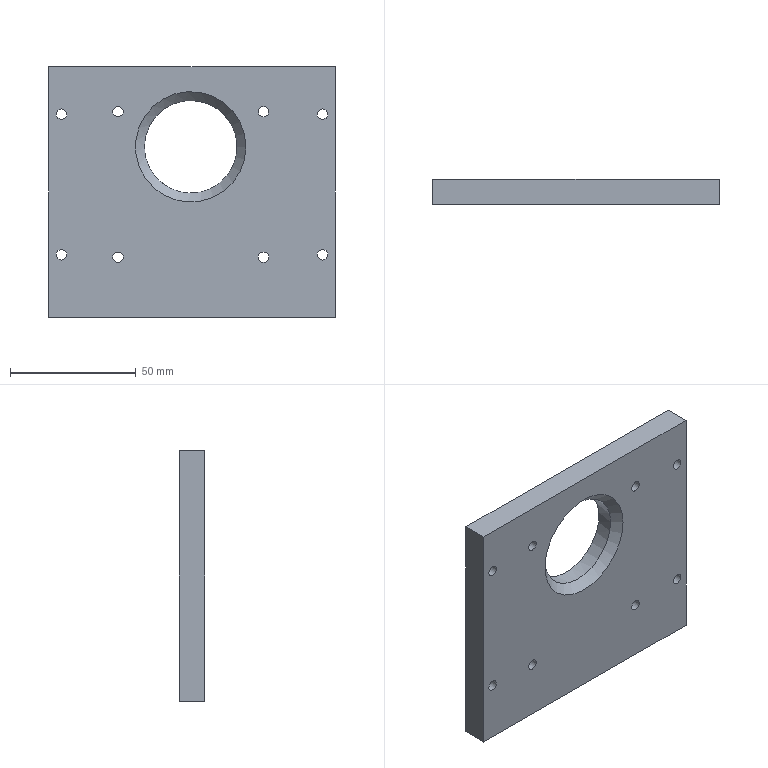Part | STEP file | ROTATION MC_NEW VER-0610_980 | 1 solid | 18 faces | box 114 x 10 x 100 mm | volume 101269 mm3 | cylinder 10 | plane 6 | cone 2 | commonest cylinder face diameters 4.134 x4 4.2 x4 3.3 x1 37 x1
STEP:
#1=CARTESIAN_POINT('',(-288.528,683.508,-245.083));
#2=VERTEX_POINT('',#1);
#3=CARTESIAN_POINT('',(-286.461,683.508,-245.083));
#4=DIRECTION('',(0.,-1.,0.));
#5=DIRECTION('',(1.,0.,0.));
#6=AXIS2_PLACEMENT_3D('',#3,#4,#5);
#7=CIRCLE('',#6,2.067);
#8=EDGE_CURVE('',#2,#2,#7,.T.);
#9=ORIENTED_EDGE('',*,*,#8,.F.);
#10=CARTESIAN_POINT('',(-288.528,673.508,-245.083));
#11=VERTEX_POINT('',#10);
#12=CARTESIAN_POINT('',(-288.528,825.482,-245.083));
#13=DIRECTION('',(0.,-1.,0.));
#14=VECTOR('',#13,2.067);
#15=LINE('',#12,#14);
#16=EDGE_CURVE('',#2,#11,#15,.T.);
#17=ORIENTED_EDGE('',*,*,#16,.T.);
#18=CARTESIAN_POINT('',(-284.394,673.508,-245.083));
#19=VERTEX_POINT('',#18);
#20=CARTESIAN_POINT('',(-286.461,673.508,-245.083));
#21=DIRECTION('',(0.,1.,0.));
#22=DIRECTION('',(1.,0.,0.));
#23=AXIS2_PLACEMENT_3D('',#20,#21,#22);
#24=CIRCLE('',#23,2.067);
#25=EDGE_CURVE('',#19,#11,#24,.T.);
#26=ORIENTED_EDGE('',*,*,#25,.F.);
#27=CARTESIAN_POINT('',(-286.461,673.508,-245.083));
#28=DIRECTION('',(0.,1.,0.));
#29=DIRECTION('',(1.,0.,0.));
#30=AXIS2_PLACEMENT_3D('',#27,#28,#29);
#31=CIRCLE('',#30,2.067);
#32=EDGE_CURVE('',#11,#19,#31,.T.);
#33=ORIENTED_EDGE('',*,*,#32,.F.);
#34=ORIENTED_EDGE('',*,*,#16,.F.);
#35=EDGE_LOOP('',(#9,#17,#26,#33,#34));
#36=FACE_OUTER_BOUND('',#35,.T.);
#37=CARTESIAN_POINT('',(-286.461,825.482,-245.083));
#38=DIRECTION('',(0.,-1.,0.));
#39=DIRECTION('',(1.,0.,0.));
#40=AXIS2_PLACEMENT_3D('',#37,#38,#39);
#41=CYLINDRICAL_SURFACE('',#40,2.067);
#42=ADVANCED_FACE('',(#36),#41,.F.);
#43=CARTESIAN_POINT('',(-288.528,683.508,-187.1));
#44=VERTEX_POINT('',#43);
#45=CARTESIAN_POINT('',(-286.461,683.508,-187.1));
#46=DIRECTION('',(0.,-1.,0.));
#47=DIRECTION('',(1.,0.,0.));
#48=AXIS2_PLACEMENT_3D('',#45,#46,#47);
#49=CIRCLE('',#48,2.067);
#50=EDGE_CURVE('',#44,#44,#49,.T.);
#51=ORIENTED_EDGE('',*,*,#50,.F.);
#52=CARTESIAN_POINT('',(-288.528,673.508,-187.1));
#53=VERTEX_POINT('',#52);
#54=CARTESIAN_POINT('',(-288.528,825.482,-187.1));
#55=DIRECTION('',(0.,-1.,0.));
#56=VECTOR('',#55,2.067);
#57=LINE('',#54,#56);
#58=EDGE_CURVE('',#44,#53,#57,.T.);
#59=ORIENTED_EDGE('',*,*,#58,.T.);
#60=CARTESIAN_POINT('',(-284.394,673.508,-187.1));
#61=VERTEX_POINT('',#60);
#62=CARTESIAN_POINT('',(-286.461,673.508,-187.1));
#63=DIRECTION('',(0.,1.,0.));
#64=DIRECTION('',(1.,0.,0.));
#65=AXIS2_PLACEMENT_3D('',#62,#63,#64);
#66=CIRCLE('',#65,2.067);
#67=EDGE_CURVE('',#61,#53,#66,.T.);
#68=ORIENTED_EDGE('',*,*,#67,.F.);
#69=CARTESIAN_POINT('',(-286.461,673.508,-187.1));
#70=DIRECTION('',(0.,1.,0.));
#71=DIRECTION('',(1.,0.,0.));
#72=AXIS2_PLACEMENT_3D('',#69,#70,#71);
#73=CIRCLE('',#72,2.067);
#74=EDGE_CURVE('',#53,#61,#73,.T.);
#75=ORIENTED_EDGE('',*,*,#74,.F.);
#76=ORIENTED_EDGE('',*,*,#58,.F.);
#77=EDGE_LOOP('',(#51,#59,#68,#75,#76));
#78=FACE_OUTER_BOUND('',#77,.T.);
#79=CARTESIAN_POINT('',(-286.461,825.482,-187.1));
#80=DIRECTION('',(0.,-1.,0.));
#81=DIRECTION('',(1.,0.,0.));
#82=AXIS2_PLACEMENT_3D('',#79,#80,#81);
#83=CYLINDRICAL_SURFACE('',#82,2.067);
#84=ADVANCED_FACE('',(#78),#83,.F.);
#85=CARTESIAN_POINT('',(-230.545,683.508,-187.1));
#86=VERTEX_POINT('',#85);
#87=CARTESIAN_POINT('',(-228.478,683.508,-187.1));
#88=DIRECTION('',(0.,-1.,0.));
#89=DIRECTION('',(1.,0.,0.));
#90=AXIS2_PLACEMENT_3D('',#87,#88,#89);
#91=CIRCLE('',#90,2.067);
#92=EDGE_CURVE('',#86,#86,#91,.T.);
#93=ORIENTED_EDGE('',*,*,#92,.F.);
#94=CARTESIAN_POINT('',(-230.545,673.508,-187.1));
#95=VERTEX_POINT('',#94);
#96=CARTESIAN_POINT('',(-230.545,825.482,-187.1));
#97=DIRECTION('',(0.,-1.,0.));
#98=VECTOR('',#97,2.067);
#99=LINE('',#96,#98);
#100=EDGE_CURVE('',#86,#95,#99,.T.);
#101=ORIENTED_EDGE('',*,*,#100,.T.);
#102=CARTESIAN_POINT('',(-226.411,673.508,-187.1));
#103=VERTEX_POINT('',#102);
#104=CARTESIAN_POINT('',(-228.478,673.508,-187.1));
#105=DIRECTION('',(0.,1.,0.));
#106=DIRECTION('',(1.,0.,0.));
#107=AXIS2_PLACEMENT_3D('',#104,#105,#106);
#108=CIRCLE('',#107,2.067);
#109=EDGE_CURVE('',#103,#95,#108,.T.);
#110=ORIENTED_EDGE('',*,*,#109,.F.);
#111=CARTESIAN_POINT('',(-228.478,673.508,-187.1));
#112=DIRECTION('',(0.,1.,0.));
#113=DIRECTION('',(1.,0.,0.));
#114=AXIS2_PLACEMENT_3D('',#111,#112,#113);
#115=CIRCLE('',#114,2.067);
#116=EDGE_CURVE('',#95,#103,#115,.T.);
#117=ORIENTED_EDGE('',*,*,#116,.F.);
#118=ORIENTED_EDGE('',*,*,#100,.F.);
#119=EDGE_LOOP('',(#93,#101,#110,#117,#118));
#120=FACE_OUTER_BOUND('',#119,.T.);
#121=CARTESIAN_POINT('',(-228.478,825.482,-187.1));
#122=DIRECTION('',(0.,-1.,0.));
#123=DIRECTION('',(1.,0.,0.));
#124=AXIS2_PLACEMENT_3D('',#121,#122,#123);
#125=CYLINDRICAL_SURFACE('',#124,2.067);
#126=ADVANCED_FACE('',(#120),#125,.F.);
#127=CARTESIAN_POINT('',(-230.545,683.508,-245.083));
#128=VERTEX_POINT('',#127);
#129=CARTESIAN_POINT('',(-228.478,683.508,-245.083));
#130=DIRECTION('',(0.,-1.,0.));
#131=DIRECTION('',(1.,0.,0.));
#132=AXIS2_PLACEMENT_3D('',#129,#130,#131);
#133=CIRCLE('',#132,2.067);
#134=EDGE_CURVE('',#128,#128,#133,.T.);
#135=ORIENTED_EDGE('',*,*,#134,.F.);
#136=CARTESIAN_POINT('',(-230.545,673.508,-245.083));
#137=VERTEX_POINT('',#136);
#138=CARTESIAN_POINT('',(-230.545,825.482,-245.083));
#139=DIRECTION('',(0.,-1.,0.));
#140=VECTOR('',#139,2.067);
#141=LINE('',#138,#140);
#142=EDGE_CURVE('',#128,#137,#141,.T.);
#143=ORIENTED_EDGE('',*,*,#142,.T.);
#144=CARTESIAN_POINT('',(-226.411,673.508,-245.083));
#145=VERTEX_POINT('',#144);
#146=CARTESIAN_POINT('',(-228.478,673.508,-245.083));
#147=DIRECTION('',(0.,1.,0.));
#148=DIRECTION('',(1.,0.,0.));
#149=AXIS2_PLACEMENT_3D('',#146,#147,#148);
#150=CIRCLE('',#149,2.067);
#151=EDGE_CURVE('',#145,#137,#150,.T.);
#152=ORIENTED_EDGE('',*,*,#151,.F.);
#153=CARTESIAN_POINT('',(-228.478,673.508,-245.083));
#154=DIRECTION('',(0.,1.,0.));
#155=DIRECTION('',(1.,0.,0.));
#156=AXIS2_PLACEMENT_3D('',#153,#154,#155);
#157=CIRCLE('',#156,2.067);
#158=EDGE_CURVE('',#137,#145,#157,.T.);
#159=ORIENTED_EDGE('',*,*,#158,.F.);
#160=ORIENTED_EDGE('',*,*,#142,.F.);
#161=EDGE_LOOP('',(#135,#143,#152,#159,#160));
#162=FACE_OUTER_BOUND('',#161,.T.);
#163=CARTESIAN_POINT('',(-228.478,825.482,-245.083));
#164=DIRECTION('',(0.,-1.,0.));
#165=DIRECTION('',(1.,0.,0.));
#166=AXIS2_PLACEMENT_3D('',#163,#164,#165);
#167=CYLINDRICAL_SURFACE('',#166,2.067);
#168=ADVANCED_FACE('',(#162),#167,.F.);
#169=CARTESIAN_POINT('',(-308.969,683.508,-185.991));
#170=VERTEX_POINT('',#169);
#171=CARTESIAN_POINT('',(-308.969,683.508,-188.091));
#172=DIRECTION('',(0.,1.,0.));
#173=DIRECTION('',(0.,0.,1.));
#174=AXIS2_PLACEMENT_3D('',#171,#172,#173);
#175=CIRCLE('',#174,2.1);
#176=EDGE_CURVE('',#170,#170,#175,.F.);
#177=ORIENTED_EDGE('',*,*,#176,.F.);
#178=CARTESIAN_POINT('',(-308.969,673.508,-185.991));
#179=VERTEX_POINT('',#178);
#180=CARTESIAN_POINT('',(-308.969,683.508,-185.991));
#181=DIRECTION('',(0.,-1.,0.));
#182=VECTOR('',#181,2.1);
#183=LINE('',#180,#182);
#184=EDGE_CURVE('',#170,#179,#183,.T.);
#185=ORIENTED_EDGE('',*,*,#184,.T.);
#186=CARTESIAN_POINT('',(-308.969,673.508,-188.091));
#187=DIRECTION('',(0.,1.,0.));
#188=DIRECTION('',(0.,0.,1.));
#189=AXIS2_PLACEMENT_3D('',#186,#187,#188);
#190=CIRCLE('',#189,2.1);
#191=EDGE_CURVE('',#179,#179,#190,.T.);
#192=ORIENTED_EDGE('',*,*,#191,.F.);
#193=ORIENTED_EDGE('',*,*,#184,.F.);
#194=EDGE_LOOP('',(#177,#185,#192,#193));
#195=FACE_OUTER_BOUND('',#194,.T.);
#196=CARTESIAN_POINT('',(-308.969,683.508,-188.091));
#197=DIRECTION('',(0.,-1.,0.));
#198=DIRECTION('',(0.,0.,-1.));
#199=AXIS2_PLACEMENT_3D('',#196,#197,#198);
#200=CYLINDRICAL_SURFACE('',#199,2.1);
#201=ADVANCED_FACE('',(#195),#200,.F.);
#202=CARTESIAN_POINT('',(-308.969,683.508,-241.991));
#203=VERTEX_POINT('',#202);
#204=CARTESIAN_POINT('',(-308.969,683.508,-244.091));
#205=DIRECTION('',(0.,1.,0.));
#206=DIRECTION('',(0.,0.,1.));
#207=AXIS2_PLACEMENT_3D('',#204,#205,#206);
#208=CIRCLE('',#207,2.1);
#209=EDGE_CURVE('',#203,#203,#208,.F.);
#210=ORIENTED_EDGE('',*,*,#209,.F.);
#211=CARTESIAN_POINT('',(-308.969,673.508,-241.991));
#212=VERTEX_POINT('',#211);
#213=CARTESIAN_POINT('',(-308.969,683.508,-241.991));
#214=DIRECTION('',(0.,-1.,0.));
#215=VECTOR('',#214,2.1);
#216=LINE('',#213,#215);
#217=EDGE_CURVE('',#203,#212,#216,.T.);
#218=ORIENTED_EDGE('',*,*,#217,.T.);
#219=CARTESIAN_POINT('',(-308.969,673.508,-244.091));
#220=DIRECTION('',(0.,1.,0.));
#221=DIRECTION('',(0.,0.,1.));
#222=AXIS2_PLACEMENT_3D('',#219,#220,#221);
#223=CIRCLE('',#222,2.1);
#224=EDGE_CURVE('',#212,#212,#223,.T.);
#225=ORIENTED_EDGE('',*,*,#224,.F.);
#226=ORIENTED_EDGE('',*,*,#217,.F.);
#227=EDGE_LOOP('',(#210,#218,#225,#226));
#228=FACE_OUTER_BOUND('',#227,.T.);
#229=CARTESIAN_POINT('',(-308.969,683.508,-244.091));
#230=DIRECTION('',(0.,-1.,0.));
#231=DIRECTION('',(0.,0.,-1.));
#232=AXIS2_PLACEMENT_3D('',#229,#230,#231);
#233=CYLINDRICAL_SURFACE('',#232,2.1);
#234=ADVANCED_FACE('',(#228),#233,.F.);
#235=CARTESIAN_POINT('',(-204.969,683.508,-241.991));
#236=VERTEX_POINT('',#235);
#237=CARTESIAN_POINT('',(-204.969,683.508,-244.091));
#238=DIRECTION('',(0.,1.,0.));
#239=DIRECTION('',(0.,0.,1.));
#240=AXIS2_PLACEMENT_3D('',#237,#238,#239);
#241=CIRCLE('',#240,2.1);
#242=EDGE_CURVE('',#236,#236,#241,.F.);
#243=ORIENTED_EDGE('',*,*,#242,.F.);
#244=CARTESIAN_POINT('',(-204.969,673.508,-241.991));
#245=VERTEX_POINT('',#244);
#246=CARTESIAN_POINT('',(-204.969,683.508,-241.991));
#247=DIRECTION('',(0.,-1.,0.));
#248=VECTOR('',#247,2.1);
#249=LINE('',#246,#248);
#250=EDGE_CURVE('',#236,#245,#249,.T.);
#251=ORIENTED_EDGE('',*,*,#250,.T.);
#252=CARTESIAN_POINT('',(-204.969,673.508,-244.091));
#253=DIRECTION('',(0.,1.,0.));
#254=DIRECTION('',(0.,0.,1.));
#255=AXIS2_PLACEMENT_3D('',#252,#253,#254);
#256=CIRCLE('',#255,2.1);
#257=EDGE_CURVE('',#245,#245,#256,.T.);
#258=ORIENTED_EDGE('',*,*,#257,.F.);
#259=ORIENTED_EDGE('',*,*,#250,.F.);
#260=EDGE_LOOP('',(#243,#251,#258,#259));
#261=FACE_OUTER_BOUND('',#260,.T.);
#262=CARTESIAN_POINT('',(-204.969,683.508,-244.091));
#263=DIRECTION('',(0.,-1.,0.));
#264=DIRECTION('',(0.,0.,-1.));
#265=AXIS2_PLACEMENT_3D('',#262,#263,#264);
#266=CYLINDRICAL_SURFACE('',#265,2.1);
#267=ADVANCED_FACE('',(#261),#266,.F.);
#268=CARTESIAN_POINT('',(-204.969,683.508,-185.991));
#269=VERTEX_POINT('',#268);
#270=CARTESIAN_POINT('',(-204.969,683.508,-188.091));
#271=DIRECTION('',(0.,1.,0.));
#272=DIRECTION('',(0.,0.,1.));
#273=AXIS2_PLACEMENT_3D('',#270,#271,#272);
#274=CIRCLE('',#273,2.1);
#275=EDGE_CURVE('',#269,#269,#274,.F.);
#276=ORIENTED_EDGE('',*,*,#275,.F.);
#277=CARTESIAN_POINT('',(-204.969,673.508,-185.991));
#278=VERTEX_POINT('',#277);
#279=CARTESIAN_POINT('',(-204.969,683.508,-185.991));
#280=DIRECTION('',(0.,-1.,0.));
#281=VECTOR('',#280,2.1);
#282=LINE('',#279,#281);
#283=EDGE_CURVE('',#269,#278,#282,.T.);
#284=ORIENTED_EDGE('',*,*,#283,.T.);
#285=CARTESIAN_POINT('',(-204.969,673.508,-188.091));
#286=DIRECTION('',(0.,1.,0.));
#287=DIRECTION('',(0.,0.,1.));
#288=AXIS2_PLACEMENT_3D('',#285,#286,#287);
#289=CIRCLE('',#288,2.1);
#290=EDGE_CURVE('',#278,#278,#289,.T.);
#291=ORIENTED_EDGE('',*,*,#290,.F.);
#292=ORIENTED_EDGE('',*,*,#283,.F.);
#293=EDGE_LOOP('',(#276,#284,#291,#292));
#294=FACE_OUTER_BOUND('',#293,.T.);
#295=CARTESIAN_POINT('',(-204.969,683.508,-188.091));
#296=DIRECTION('',(0.,-1.,0.));
#297=DIRECTION('',(0.,0.,-1.));
#298=AXIS2_PLACEMENT_3D('',#295,#296,#297);
#299=CYLINDRICAL_SURFACE('',#298,2.1);
#300=ADVANCED_FACE('',(#294),#299,.F.);
#301=CARTESIAN_POINT('',(-256.969,678.358,-269.091));
#302=VERTEX_POINT('',#301);
#303=CARTESIAN_POINT('',(-256.969,681.658,-269.091));
#304=VERTEX_POINT('',#303);
#305=CARTESIAN_POINT('',(-256.969,680.008,-269.091));
#306=DIRECTION('',(0.,0.,1.));
#307=DIRECTION('',(0.,-1.,0.));
#308=AXIS2_PLACEMENT_3D('',#305,#306,#307);
#309=CIRCLE('',#308,1.65);
#310=EDGE_CURVE('',#302,#304,#309,.T.);
#311=ORIENTED_EDGE('',*,*,#310,.F.);
#312=CARTESIAN_POINT('',(-256.969,680.008,-269.091));
#313=DIRECTION('',(0.,0.,1.));
#314=DIRECTION('',(0.,-1.,0.));
#315=AXIS2_PLACEMENT_3D('',#312,#313,#314);
#316=CIRCLE('',#315,1.65);
#317=EDGE_CURVE('',#304,#302,#316,.T.);
#318=ORIENTED_EDGE('',*,*,#317,.F.);
#319=CARTESIAN_POINT('',(-256.969,681.658,-254.091));
#320=VERTEX_POINT('',#319);
#321=CARTESIAN_POINT('',(-256.969,681.658,-269.091));
#322=DIRECTION('',(0.,0.,1.));
#323=VECTOR('',#322,1.65);
#324=LINE('',#321,#323);
#325=EDGE_CURVE('',#304,#320,#324,.T.);
#326=ORIENTED_EDGE('',*,*,#325,.T.);
#327=CARTESIAN_POINT('',(-256.969,678.358,-254.091));
#328=VERTEX_POINT('',#327);
#329=CARTESIAN_POINT('',(-256.969,680.008,-254.091));
#330=DIRECTION('',(0.,0.,-1.));
#331=DIRECTION('',(0.,-1.,0.));
#332=AXIS2_PLACEMENT_3D('',#329,#330,#331);
#333=CIRCLE('',#332,1.65);
#334=EDGE_CURVE('',#328,#320,#333,.T.);
#335=ORIENTED_EDGE('',*,*,#334,.F.);
#336=CARTESIAN_POINT('',(-256.969,680.008,-254.091));
#337=DIRECTION('',(0.,0.,-1.));
#338=DIRECTION('',(0.,-1.,0.));
#339=AXIS2_PLACEMENT_3D('',#336,#337,#338);
#340=CIRCLE('',#339,1.65);
#341=EDGE_CURVE('',#320,#328,#340,.T.);
#342=ORIENTED_EDGE('',*,*,#341,.F.);
#343=ORIENTED_EDGE('',*,*,#325,.F.);
#344=EDGE_LOOP('',(#311,#318,#326,#335,#342,#343));
#345=FACE_OUTER_BOUND('',#344,.T.);
#346=CARTESIAN_POINT('',(-256.969,680.008,-269.091));
#347=DIRECTION('',(0.,0.,1.));
#348=DIRECTION('',(0.,-1.,0.));
#349=AXIS2_PLACEMENT_3D('',#346,#347,#348);
#350=CYLINDRICAL_SURFACE('',#349,1.65);
#351=ADVANCED_FACE('',(#345),#350,.F.);
#352=CARTESIAN_POINT('',(-256.969,680.008,-253.1));
#353=VERTEX_POINT('',#352);
#354=CARTESIAN_POINT('',(-256.969,678.358,-254.091));
#355=DIRECTION('',(0.,-0.8572,-0.515));
#356=VECTOR('',#355,1.65);
#357=LINE('',#354,#356);
#358=EDGE_CURVE('',#353,#328,#357,.T.);
#359=ORIENTED_EDGE('',*,*,#358,.T.);
#360=ORIENTED_EDGE('',*,*,#334,.T.);
#361=ORIENTED_EDGE('',*,*,#341,.T.);
#362=ORIENTED_EDGE('',*,*,#358,.F.);
#363=EDGE_LOOP('',(#359,#360,#361,#362));
#364=FACE_OUTER_BOUND('',#363,.T.);
#365=CARTESIAN_POINT('',(-256.969,680.008,-254.091));
#366=DIRECTION('',(0.,0.,-1.));
#367=DIRECTION('',(0.,1.,0.));
#368=AXIS2_PLACEMENT_3D('',#365,#366,#367);
#369=CONICAL_SURFACE('',#368,1.65,1.03);
#370=ADVANCED_FACE('',(#364),#369,.F.);
#371=CARTESIAN_POINT('',(-199.969,673.508,-269.091));
#372=VERTEX_POINT('',#371);
#373=CARTESIAN_POINT('',(-313.969,673.508,-269.091));
#374=VERTEX_POINT('',#373);
#375=CARTESIAN_POINT('',(-199.969,673.508,-269.091));
#376=DIRECTION('',(-1.,0.,0.));
#377=VECTOR('',#376,114.);
#378=LINE('',#375,#377);
#379=EDGE_CURVE('',#372,#374,#378,.T.);
#380=ORIENTED_EDGE('',*,*,#379,.T.);
#381=CARTESIAN_POINT('',(-313.969,683.508,-269.091));
#382=VERTEX_POINT('',#381);
#383=CARTESIAN_POINT('',(-313.969,683.508,-269.091));
#384=DIRECTION('',(0.,-1.,0.));
#385=VECTOR('',#384,10.);
#386=LINE('',#383,#385);
#387=EDGE_CURVE('',#382,#374,#386,.T.);
#388=ORIENTED_EDGE('',*,*,#387,.F.);
#389=CARTESIAN_POINT('',(-199.969,683.508,-269.091));
#390=VERTEX_POINT('',#389);
#391=CARTESIAN_POINT('',(-199.969,683.508,-269.091));
#392=DIRECTION('',(-1.,0.,0.));
#393=VECTOR('',#392,114.);
#394=LINE('',#391,#393);
#395=EDGE_CURVE('',#390,#382,#394,.T.);
#396=ORIENTED_EDGE('',*,*,#395,.F.);
#397=CARTESIAN_POINT('',(-199.969,683.508,-269.091));
#398=DIRECTION('',(0.,-1.,0.));
#399=VECTOR('',#398,10.);
#400=LINE('',#397,#399);
#401=EDGE_CURVE('',#390,#372,#400,.T.);
#402=ORIENTED_EDGE('',*,*,#401,.T.);
#403=EDGE_LOOP('',(#380,#388,#396,#402));
#404=FACE_OUTER_BOUND('',#403,.T.);
#405=ORIENTED_EDGE('',*,*,#310,.T.);
#406=ORIENTED_EDGE('',*,*,#317,.T.);
#407=EDGE_LOOP('',(#405,#406));
#408=FACE_BOUND('',#407,.T.);
#409=CARTESIAN_POINT('',(-258.469,676.508,-269.091));
#410=DIRECTION('',(0.,0.,-1.));
#411=DIRECTION('',(-1.,0.,0.));
#412=AXIS2_PLACEMENT_3D('',#409,#410,#411);
#413=PLANE('',#412);
#414=ADVANCED_FACE('',(#404,#408),#413,.T.);
#415=CARTESIAN_POINT('',(-313.969,683.508,-169.091));
#416=VERTEX_POINT('',#415);
#417=CARTESIAN_POINT('',(-313.969,683.508,-269.091));
#418=DIRECTION('',(0.,0.,1.));
#419=VECTOR('',#418,100.);
#420=LINE('',#417,#419);
#421=EDGE_CURVE('',#382,#416,#420,.T.);
#422=ORIENTED_EDGE('',*,*,#421,.T.);
#423=CARTESIAN_POINT('',(-199.969,683.508,-169.091));
#424=VERTEX_POINT('',#423);
#425=CARTESIAN_POINT('',(-199.969,683.508,-169.091));
#426=DIRECTION('',(-1.,0.,0.));
#427=VECTOR('',#426,114.);
#428=LINE('',#425,#427);
#429=EDGE_CURVE('',#424,#416,#428,.T.);
#430=ORIENTED_EDGE('',*,*,#429,.F.);
#431=CARTESIAN_POINT('',(-199.969,683.508,-269.091));
#432=DIRECTION('',(0.,0.,1.));
#433=VECTOR('',#432,100.);
#434=LINE('',#431,#433);
#435=EDGE_CURVE('',#390,#424,#434,.T.);
#436=ORIENTED_EDGE('',*,*,#435,.F.);
#437=ORIENTED_EDGE('',*,*,#395,.T.);
#438=EDGE_LOOP('',(#422,#430,#436,#437));
#439=FACE_OUTER_BOUND('',#438,.T.);
#440=ORIENTED_EDGE('',*,*,#8,.T.);
#441=EDGE_LOOP('',(#440));
#442=FACE_BOUND('',#441,.T.);
#443=ORIENTED_EDGE('',*,*,#50,.T.);
#444=EDGE_LOOP('',(#443));
#445=FACE_BOUND('',#444,.T.);
#446=ORIENTED_EDGE('',*,*,#92,.T.);
#447=EDGE_LOOP('',(#446));
#448=FACE_BOUND('',#447,.T.);
#449=ORIENTED_EDGE('',*,*,#134,.T.);
#450=EDGE_LOOP('',(#449));
#451=FACE_BOUND('',#450,.T.);
#452=ORIENTED_EDGE('',*,*,#275,.T.);
#453=EDGE_LOOP('',(#452));
#454=FACE_BOUND('',#453,.T.);
#455=ORIENTED_EDGE('',*,*,#242,.T.);
#456=EDGE_LOOP('',(#455));
#457=FACE_BOUND('',#456,.T.);
#458=ORIENTED_EDGE('',*,*,#209,.T.);
#459=EDGE_LOOP('',(#458));
#460=FACE_BOUND('',#459,.T.);
#461=ORIENTED_EDGE('',*,*,#176,.T.);
#462=EDGE_LOOP('',(#461));
#463=FACE_BOUND('',#462,.T.);
#464=CARTESIAN_POINT('',(-257.469,683.508,-182.591));
#465=VERTEX_POINT('',#464);
#466=CARTESIAN_POINT('',(-275.969,683.508,-201.091));
#467=VERTEX_POINT('',#466);
#468=CARTESIAN_POINT('',(-257.469,683.508,-201.091));
#469=DIRECTION('',(0.,-1.,0.));
#470=DIRECTION('',(0.,0.,1.));
#471=AXIS2_PLACEMENT_3D('',#468,#469,#470);
#472=CIRCLE('',#471,18.5);
#473=EDGE_CURVE('',#465,#467,#472,.T.);
#474=ORIENTED_EDGE('',*,*,#473,.T.);
#475=CARTESIAN_POINT('',(-257.469,683.508,-201.091));
#476=DIRECTION('',(0.,-1.,0.));
#477=DIRECTION('',(0.,0.,1.));
#478=AXIS2_PLACEMENT_3D('',#475,#476,#477);
#479=CIRCLE('',#478,18.5);
#480=EDGE_CURVE('',#467,#465,#479,.T.);
#481=ORIENTED_EDGE('',*,*,#480,.T.);
#482=EDGE_LOOP('',(#474,#481));
#483=FACE_BOUND('',#482,.T.);
#484=CARTESIAN_POINT('',(-257.469,683.508,-228.812));
#485=DIRECTION('',(0.,1.,0.));
#486=DIRECTION('',(0.,0.,1.));
#487=AXIS2_PLACEMENT_3D('',#484,#485,#486);
#488=PLANE('',#487);
#489=ADVANCED_FACE('',(#439,#442,#445,#448,#451,#454,#457,#460,#463,#483),#488,.T.);
#490=CARTESIAN_POINT('',(-313.969,673.508,-169.091));
#491=VERTEX_POINT('',#490);
#492=CARTESIAN_POINT('',(-199.969,673.508,-169.091));
#493=VERTEX_POINT('',#492);
#494=CARTESIAN_POINT('',(-313.969,673.508,-169.091));
#495=DIRECTION('',(1.,0.,0.));
#496=VECTOR('',#495,114.);
#497=LINE('',#494,#496);
#498=EDGE_CURVE('',#491,#493,#497,.T.);
#499=ORIENTED_EDGE('',*,*,#498,.F.);
#500=CARTESIAN_POINT('',(-313.969,673.508,-269.091));
#501=DIRECTION('',(0.,0.,1.));
#502=VECTOR('',#501,100.);
#503=LINE('',#500,#502);
#504=EDGE_CURVE('',#374,#491,#503,.T.);
#505=ORIENTED_EDGE('',*,*,#504,.F.);
#506=ORIENTED_EDGE('',*,*,#379,.F.);
#507=CARTESIAN_POINT('',(-199.969,673.508,-169.091));
#508=DIRECTION('',(0.,0.,-1.));
#509=VECTOR('',#508,100.);
#510=LINE('',#507,#509);
#511=EDGE_CURVE('',#493,#372,#510,.T.);
#512=ORIENTED_EDGE('',*,*,#511,.F.);
#513=EDGE_LOOP('',(#499,#505,#506,#512));
#514=FACE_OUTER_BOUND('',#513,.T.);
#515=ORIENTED_EDGE('',*,*,#25,.T.);
#516=ORIENTED_EDGE('',*,*,#32,.T.);
#517=EDGE_LOOP('',(#515,#516));
#518=FACE_BOUND('',#517,.T.);
#519=ORIENTED_EDGE('',*,*,#67,.T.);
#520=ORIENTED_EDGE('',*,*,#74,.T.);
#521=EDGE_LOOP('',(#519,#520));
#522=FACE_BOUND('',#521,.T.);
#523=ORIENTED_EDGE('',*,*,#109,.T.);
#524=ORIENTED_EDGE('',*,*,#116,.T.);
#525=EDGE_LOOP('',(#523,#524));
#526=FACE_BOUND('',#525,.T.);
#527=ORIENTED_EDGE('',*,*,#151,.T.);
#528=ORIENTED_EDGE('',*,*,#158,.T.);
#529=EDGE_LOOP('',(#527,#528));
#530=FACE_BOUND('',#529,.T.);
#531=CARTESIAN_POINT('',(-235.469,673.508,-201.091));
#532=VERTEX_POINT('',#531);
#533=CARTESIAN_POINT('',(-257.469,673.508,-201.091));
#534=DIRECTION('',(0.,1.,0.));
#535=DIRECTION('',(-1.,0.,0.));
#536=AXIS2_PLACEMENT_3D('',#533,#534,#535);
#537=CIRCLE('',#536,22.);
#538=EDGE_CURVE('',#532,#532,#537,.T.);
#539=ORIENTED_EDGE('',*,*,#538,.T.);
#540=EDGE_LOOP('',(#539));
#541=FACE_BOUND('',#540,.T.);
#542=ORIENTED_EDGE('',*,*,#290,.T.);
#543=EDGE_LOOP('',(#542));
#544=FACE_BOUND('',#543,.T.);
#545=ORIENTED_EDGE('',*,*,#257,.T.);
#546=EDGE_LOOP('',(#545));
#547=FACE_BOUND('',#546,.T.);
#548=ORIENTED_EDGE('',*,*,#224,.T.);
#549=EDGE_LOOP('',(#548));
#550=FACE_BOUND('',#549,.T.);
#551=ORIENTED_EDGE('',*,*,#191,.T.);
#552=EDGE_LOOP('',(#551));
#553=FACE_BOUND('',#552,.T.);
#554=CARTESIAN_POINT('',(-257.469,673.508,-216.091));
#555=DIRECTION('',(0.,1.,0.));
#556=DIRECTION('',(0.,0.,1.));
#557=AXIS2_PLACEMENT_3D('',#554,#555,#556);
#558=PLANE('',#557);
#559=ADVANCED_FACE('',(#514,#518,#522,#526,#530,#541,#544,#547,#550,#553),#558,.F.);
#560=ORIENTED_EDGE('',*,*,#421,.F.);
#561=ORIENTED_EDGE('',*,*,#387,.T.);
#562=ORIENTED_EDGE('',*,*,#504,.T.);
#563=CARTESIAN_POINT('',(-313.969,673.508,-169.091));
#564=DIRECTION('',(0.,1.,0.));
#565=VECTOR('',#564,10.);
#566=LINE('',#563,#565);
#567=EDGE_CURVE('',#491,#416,#566,.T.);
#568=ORIENTED_EDGE('',*,*,#567,.T.);
#569=EDGE_LOOP('',(#560,#561,#562,#568));
#570=FACE_OUTER_BOUND('',#569,.T.);
#571=CARTESIAN_POINT('',(-313.969,676.508,-228.812));
#572=DIRECTION('',(-1.,0.,0.));
#573=DIRECTION('',(0.,0.,1.));
#574=AXIS2_PLACEMENT_3D('',#571,#572,#573);
#575=PLANE('',#574);
#576=ADVANCED_FACE('',(#570),#575,.T.);
#577=ORIENTED_EDGE('',*,*,#498,.T.);
#578=CARTESIAN_POINT('',(-199.969,673.508,-169.091));
#579=DIRECTION('',(0.,1.,0.));
#580=VECTOR('',#579,10.);
#581=LINE('',#578,#580);
#582=EDGE_CURVE('',#493,#424,#581,.T.);
#583=ORIENTED_EDGE('',*,*,#582,.T.);
#584=ORIENTED_EDGE('',*,*,#429,.T.);
#585=ORIENTED_EDGE('',*,*,#567,.F.);
#586=EDGE_LOOP('',(#577,#583,#584,#585));
#587=FACE_OUTER_BOUND('',#586,.T.);
#588=CARTESIAN_POINT('',(-258.469,676.508,-169.091));
#589=DIRECTION('',(0.,0.,1.));
#590=DIRECTION('',(1.,0.,0.));
#591=AXIS2_PLACEMENT_3D('',#588,#589,#590);
#592=PLANE('',#591);
#593=ADVANCED_FACE('',(#587),#592,.T.);
#594=ORIENTED_EDGE('',*,*,#511,.T.);
#595=ORIENTED_EDGE('',*,*,#401,.F.);
#596=ORIENTED_EDGE('',*,*,#435,.T.);
#597=ORIENTED_EDGE('',*,*,#582,.F.);
#598=EDGE_LOOP('',(#594,#595,#596,#597));
#599=FACE_OUTER_BOUND('',#598,.T.);
#600=CARTESIAN_POINT('',(-199.969,676.508,-228.812));
#601=DIRECTION('',(1.,0.,0.));
#602=DIRECTION('',(0.,0.,-1.));
#603=AXIS2_PLACEMENT_3D('',#600,#601,#602);
#604=PLANE('',#603);
#605=ADVANCED_FACE('',(#599),#604,.T.);
#606=CARTESIAN_POINT('',(-257.469,677.008,-219.591));
#607=VERTEX_POINT('',#606);
#608=CARTESIAN_POINT('',(-275.969,677.008,-201.091));
#609=VERTEX_POINT('',#608);
#610=CARTESIAN_POINT('',(-257.469,677.008,-201.091));
#611=DIRECTION('',(0.,1.,0.));
#612=DIRECTION('',(0.,0.,-1.));
#613=AXIS2_PLACEMENT_3D('',#610,#611,#612);
#614=CIRCLE('',#613,18.5);
#615=EDGE_CURVE('',#607,#609,#614,.T.);
#616=ORIENTED_EDGE('',*,*,#615,.T.);
#617=CARTESIAN_POINT('',(-238.969,677.008,-201.091));
#618=VERTEX_POINT('',#617);
#619=CARTESIAN_POINT('',(-257.469,677.008,-201.091));
#620=DIRECTION('',(0.,1.,0.));
#621=DIRECTION('',(0.,0.,-1.));
#622=AXIS2_PLACEMENT_3D('',#619,#620,#621);
#623=CIRCLE('',#622,18.5);
#624=EDGE_CURVE('',#609,#618,#623,.T.);
#625=ORIENTED_EDGE('',*,*,#624,.T.);
#626=CARTESIAN_POINT('',(-256.469,694.508,-201.091));
#627=DIRECTION('',(0.7071,-0.7071,0.));
#628=VECTOR('',#627,1.);
#629=LINE('',#626,#628);
#630=EDGE_CURVE('',#618,#532,#629,.T.);
#631=ORIENTED_EDGE('',*,*,#630,.T.);
#632=ORIENTED_EDGE('',*,*,#538,.F.);
#633=ORIENTED_EDGE('',*,*,#630,.F.);
#634=CARTESIAN_POINT('',(-257.469,677.008,-201.091));
#635=DIRECTION('',(0.,1.,0.));
#636=DIRECTION('',(0.,0.,-1.));
#637=AXIS2_PLACEMENT_3D('',#634,#635,#636);
#638=CIRCLE('',#637,18.5);
#639=EDGE_CURVE('',#618,#607,#638,.T.);
#640=ORIENTED_EDGE('',*,*,#639,.T.);
#641=EDGE_LOOP('',(#616,#625,#631,#632,#633,#640));
#642=FACE_OUTER_BOUND('',#641,.T.);
#643=CARTESIAN_POINT('',(-257.469,694.508,-201.091));
#644=DIRECTION('',(0.,-1.,0.));
#645=DIRECTION('',(-1.,0.,0.));
#646=AXIS2_PLACEMENT_3D('',#643,#644,#645);
#647=CONICAL_SURFACE('',#646,1.,0.7854);
#648=ADVANCED_FACE('',(#642),#647,.F.);
#649=ORIENTED_EDGE('',*,*,#615,.F.);
#650=ORIENTED_EDGE('',*,*,#639,.F.);
#651=ORIENTED_EDGE('',*,*,#624,.F.);
#652=CARTESIAN_POINT('',(-275.969,676.508,-201.091));
#653=DIRECTION('',(0.,1.,0.));
#654=VECTOR('',#653,18.5);
#655=LINE('',#652,#654);
#656=EDGE_CURVE('',#609,#467,#655,.T.);
#657=ORIENTED_EDGE('',*,*,#656,.T.);
#658=ORIENTED_EDGE('',*,*,#473,.F.);
#659=ORIENTED_EDGE('',*,*,#480,.F.);
#660=ORIENTED_EDGE('',*,*,#656,.F.);
#661=EDGE_LOOP('',(#649,#650,#651,#657,#658,#659,#660));
#662=FACE_OUTER_BOUND('',#661,.T.);
#663=CARTESIAN_POINT('',(-257.469,676.508,-201.091));
#664=DIRECTION('',(0.,1.,0.));
#665=DIRECTION('',(1.,0.,0.));
#666=AXIS2_PLACEMENT_3D('',#663,#664,#665);
#667=CYLINDRICAL_SURFACE('',#666,18.5);
#668=ADVANCED_FACE('',(#662),#667,.F.);
#669=CLOSED_SHELL('',(#42,#84,#126,#168,#201,#234,#267,#300,#351,#370,#414,#489,#559,#576,#593,#605,#648,#668));
#670=MANIFOLD_SOLID_BREP('',#669);
#671=(LENGTH_UNIT()NAMED_UNIT(*)SI_UNIT(.MILLI.,.METRE.));
#672=UNCERTAINTY_MEASURE_WITH_UNIT(LENGTH_MEASURE(0.01),#671,'','');
#673=(NAMED_UNIT(*)PLANE_ANGLE_UNIT()SI_UNIT($,.RADIAN.));
#674=(NAMED_UNIT(*)SI_UNIT($,.STERADIAN.)SOLID_ANGLE_UNIT());
#675=(GEOMETRIC_REPRESENTATION_CONTEXT(3)GLOBAL_UNCERTAINTY_ASSIGNED_CONTEXT((#672))GLOBAL_UNIT_ASSIGNED_CONTEXT((#671,#673,#674))REPRESENTATION_CONTEXT('',''));
#676=ADVANCED_BREP_SHAPE_REPRESENTATION('',(#670),#675);